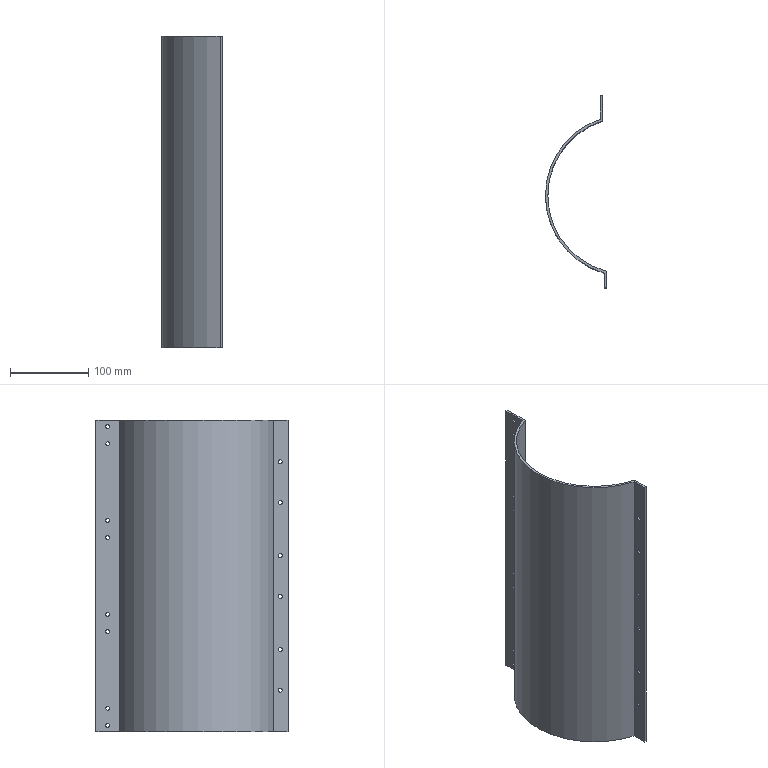Part | SolidWorks | features BaseBody 1 | 1 solid | 39 faces | box 78 x 245.57 x 398 mm | volume 370674 mm3 | cylinder 31 | plane 8 | commonest cylinder face diameters 5 x28 200 x2 206 x1
STEP:
#1=CARTESIAN_POINT('',(-30.,112.57,-365.5));
#2=VERTEX_POINT('',#1);
#3=CARTESIAN_POINT('',(-30.,112.57,-370.5));
#4=VERTEX_POINT('',#3);
#5=CARTESIAN_POINT('',(-30.,112.57,-368.));
#6=DIRECTION('',(-1.,0.,0.));
#7=DIRECTION('',(0.,0.,-1.));
#8=AXIS2_PLACEMENT_3D('',#5,#6,#7);
#9=CIRCLE('',#8,2.5);
#10=EDGE_CURVE('',#2,#4,#9,.T.);
#11=ORIENTED_EDGE('',*,*,#10,.F.);
#12=CARTESIAN_POINT('',(-33.,112.57,-365.5));
#13=VERTEX_POINT('',#12);
#14=CARTESIAN_POINT('',(-33.,112.57,-365.5));
#15=DIRECTION('',(-1.,0.,0.));
#16=VECTOR('',#15,1000.);
#17=LINE('',#14,#16);
#18=EDGE_CURVE('',#2,#13,#17,.T.);
#19=ORIENTED_EDGE('',*,*,#18,.T.);
#20=CARTESIAN_POINT('',(-33.,112.57,-370.5));
#21=VERTEX_POINT('',#20);
#22=CARTESIAN_POINT('',(-33.,112.57,-368.));
#23=DIRECTION('',(1.,0.,0.));
#24=DIRECTION('',(0.,0.,-1.));
#25=AXIS2_PLACEMENT_3D('',#22,#23,#24);
#26=CIRCLE('',#25,2.5);
#27=EDGE_CURVE('',#21,#13,#26,.T.);
#28=ORIENTED_EDGE('',*,*,#27,.F.);
#29=CARTESIAN_POINT('',(-33.,112.57,-370.5));
#30=DIRECTION('',(-1.,0.,0.));
#31=VECTOR('',#30,1000.);
#32=LINE('',#29,#31);
#33=EDGE_CURVE('',#4,#21,#32,.T.);
#34=ORIENTED_EDGE('',*,*,#33,.F.);
#35=EDGE_LOOP('',(#11,#19,#28,#34));
#36=FACE_OUTER_BOUND('',#35,.T.);
#37=CARTESIAN_POINT('',(-33.,112.57,-368.));
#38=DIRECTION('',(-1.,0.,0.));
#39=DIRECTION('',(0.,0.,-1.));
#40=AXIS2_PLACEMENT_3D('',#37,#38,#39);
#41=CYLINDRICAL_SURFACE('',#40,2.5);
#42=ADVANCED_FACE('',(#36),#41,.F.);
#43=CARTESIAN_POINT('',(-30.,112.57,-387.5));
#44=VERTEX_POINT('',#43);
#45=CARTESIAN_POINT('',(-30.,112.57,-392.5));
#46=VERTEX_POINT('',#45);
#47=CARTESIAN_POINT('',(-30.,112.57,-390.));
#48=DIRECTION('',(-1.,0.,0.));
#49=DIRECTION('',(0.,0.,-1.));
#50=AXIS2_PLACEMENT_3D('',#47,#48,#49);
#51=CIRCLE('',#50,2.5);
#52=EDGE_CURVE('',#44,#46,#51,.T.);
#53=ORIENTED_EDGE('',*,*,#52,.F.);
#54=CARTESIAN_POINT('',(-33.,112.57,-387.5));
#55=VERTEX_POINT('',#54);
#56=CARTESIAN_POINT('',(-33.,112.57,-387.5));
#57=DIRECTION('',(-1.,0.,0.));
#58=VECTOR('',#57,1000.);
#59=LINE('',#56,#58);
#60=EDGE_CURVE('',#44,#55,#59,.T.);
#61=ORIENTED_EDGE('',*,*,#60,.T.);
#62=CARTESIAN_POINT('',(-33.,112.57,-392.5));
#63=VERTEX_POINT('',#62);
#64=CARTESIAN_POINT('',(-33.,112.57,-390.));
#65=DIRECTION('',(1.,0.,0.));
#66=DIRECTION('',(0.,0.,-1.));
#67=AXIS2_PLACEMENT_3D('',#64,#65,#66);
#68=CIRCLE('',#67,2.5);
#69=EDGE_CURVE('',#63,#55,#68,.T.);
#70=ORIENTED_EDGE('',*,*,#69,.F.);
#71=CARTESIAN_POINT('',(-33.,112.57,-392.5));
#72=DIRECTION('',(-1.,0.,0.));
#73=VECTOR('',#72,1000.);
#74=LINE('',#71,#73);
#75=EDGE_CURVE('',#46,#63,#74,.T.);
#76=ORIENTED_EDGE('',*,*,#75,.F.);
#77=EDGE_LOOP('',(#53,#61,#70,#76));
#78=FACE_OUTER_BOUND('',#77,.T.);
#79=CARTESIAN_POINT('',(-33.,112.57,-390.));
#80=DIRECTION('',(-1.,0.,0.));
#81=DIRECTION('',(0.,0.,-1.));
#82=AXIS2_PLACEMENT_3D('',#79,#80,#81);
#83=CYLINDRICAL_SURFACE('',#82,2.5);
#84=ADVANCED_FACE('',(#78),#83,.F.);
#85=CARTESIAN_POINT('',(-30.,112.57,-245.5));
#86=VERTEX_POINT('',#85);
#87=CARTESIAN_POINT('',(-30.,112.57,-250.5));
#88=VERTEX_POINT('',#87);
#89=CARTESIAN_POINT('',(-30.,112.57,-248.));
#90=DIRECTION('',(-1.,0.,0.));
#91=DIRECTION('',(0.,0.,-1.));
#92=AXIS2_PLACEMENT_3D('',#89,#90,#91);
#93=CIRCLE('',#92,2.5);
#94=EDGE_CURVE('',#86,#88,#93,.T.);
#95=ORIENTED_EDGE('',*,*,#94,.F.);
#96=CARTESIAN_POINT('',(-33.,112.57,-245.5));
#97=VERTEX_POINT('',#96);
#98=CARTESIAN_POINT('',(-33.,112.57,-245.5));
#99=DIRECTION('',(-1.,0.,0.));
#100=VECTOR('',#99,1000.);
#101=LINE('',#98,#100);
#102=EDGE_CURVE('',#86,#97,#101,.T.);
#103=ORIENTED_EDGE('',*,*,#102,.T.);
#104=CARTESIAN_POINT('',(-33.,112.57,-250.5));
#105=VERTEX_POINT('',#104);
#106=CARTESIAN_POINT('',(-33.,112.57,-248.));
#107=DIRECTION('',(1.,0.,0.));
#108=DIRECTION('',(0.,0.,-1.));
#109=AXIS2_PLACEMENT_3D('',#106,#107,#108);
#110=CIRCLE('',#109,2.5);
#111=EDGE_CURVE('',#105,#97,#110,.T.);
#112=ORIENTED_EDGE('',*,*,#111,.F.);
#113=CARTESIAN_POINT('',(-33.,112.57,-250.5));
#114=DIRECTION('',(-1.,0.,0.));
#115=VECTOR('',#114,1000.);
#116=LINE('',#113,#115);
#117=EDGE_CURVE('',#88,#105,#116,.T.);
#118=ORIENTED_EDGE('',*,*,#117,.F.);
#119=EDGE_LOOP('',(#95,#103,#112,#118));
#120=FACE_OUTER_BOUND('',#119,.T.);
#121=CARTESIAN_POINT('',(-33.,112.57,-248.));
#122=DIRECTION('',(-1.,0.,0.));
#123=DIRECTION('',(0.,0.,-1.));
#124=AXIS2_PLACEMENT_3D('',#121,#122,#123);
#125=CYLINDRICAL_SURFACE('',#124,2.5);
#126=ADVANCED_FACE('',(#120),#125,.F.);
#127=CARTESIAN_POINT('',(-30.,112.57,-267.5));
#128=VERTEX_POINT('',#127);
#129=CARTESIAN_POINT('',(-30.,112.57,-272.5));
#130=VERTEX_POINT('',#129);
#131=CARTESIAN_POINT('',(-30.,112.57,-270.));
#132=DIRECTION('',(-1.,0.,0.));
#133=DIRECTION('',(0.,0.,-1.));
#134=AXIS2_PLACEMENT_3D('',#131,#132,#133);
#135=CIRCLE('',#134,2.5);
#136=EDGE_CURVE('',#128,#130,#135,.T.);
#137=ORIENTED_EDGE('',*,*,#136,.F.);
#138=CARTESIAN_POINT('',(-33.,112.57,-267.5));
#139=VERTEX_POINT('',#138);
#140=CARTESIAN_POINT('',(-33.,112.57,-267.5));
#141=DIRECTION('',(-1.,0.,0.));
#142=VECTOR('',#141,1000.);
#143=LINE('',#140,#142);
#144=EDGE_CURVE('',#128,#139,#143,.T.);
#145=ORIENTED_EDGE('',*,*,#144,.T.);
#146=CARTESIAN_POINT('',(-33.,112.57,-272.5));
#147=VERTEX_POINT('',#146);
#148=CARTESIAN_POINT('',(-33.,112.57,-270.));
#149=DIRECTION('',(1.,0.,0.));
#150=DIRECTION('',(0.,0.,-1.));
#151=AXIS2_PLACEMENT_3D('',#148,#149,#150);
#152=CIRCLE('',#151,2.5);
#153=EDGE_CURVE('',#147,#139,#152,.T.);
#154=ORIENTED_EDGE('',*,*,#153,.F.);
#155=CARTESIAN_POINT('',(-33.,112.57,-272.5));
#156=DIRECTION('',(-1.,0.,0.));
#157=VECTOR('',#156,1000.);
#158=LINE('',#155,#157);
#159=EDGE_CURVE('',#130,#147,#158,.T.);
#160=ORIENTED_EDGE('',*,*,#159,.F.);
#161=EDGE_LOOP('',(#137,#145,#154,#160));
#162=FACE_OUTER_BOUND('',#161,.T.);
#163=CARTESIAN_POINT('',(-33.,112.57,-270.));
#164=DIRECTION('',(-1.,0.,0.));
#165=DIRECTION('',(0.,0.,-1.));
#166=AXIS2_PLACEMENT_3D('',#163,#164,#165);
#167=CYLINDRICAL_SURFACE('',#166,2.5);
#168=ADVANCED_FACE('',(#162),#167,.F.);
#169=CARTESIAN_POINT('',(-30.,112.57,-125.5));
#170=VERTEX_POINT('',#169);
#171=CARTESIAN_POINT('',(-30.,112.57,-130.5));
#172=VERTEX_POINT('',#171);
#173=CARTESIAN_POINT('',(-30.,112.57,-128.));
#174=DIRECTION('',(-1.,0.,0.));
#175=DIRECTION('',(0.,0.,-1.));
#176=AXIS2_PLACEMENT_3D('',#173,#174,#175);
#177=CIRCLE('',#176,2.5);
#178=EDGE_CURVE('',#170,#172,#177,.T.);
#179=ORIENTED_EDGE('',*,*,#178,.F.);
#180=CARTESIAN_POINT('',(-33.,112.57,-125.5));
#181=VERTEX_POINT('',#180);
#182=CARTESIAN_POINT('',(-33.,112.57,-125.5));
#183=DIRECTION('',(-1.,0.,0.));
#184=VECTOR('',#183,1000.);
#185=LINE('',#182,#184);
#186=EDGE_CURVE('',#170,#181,#185,.T.);
#187=ORIENTED_EDGE('',*,*,#186,.T.);
#188=CARTESIAN_POINT('',(-33.,112.57,-130.5));
#189=VERTEX_POINT('',#188);
#190=CARTESIAN_POINT('',(-33.,112.57,-128.));
#191=DIRECTION('',(1.,0.,0.));
#192=DIRECTION('',(0.,0.,-1.));
#193=AXIS2_PLACEMENT_3D('',#190,#191,#192);
#194=CIRCLE('',#193,2.5);
#195=EDGE_CURVE('',#189,#181,#194,.T.);
#196=ORIENTED_EDGE('',*,*,#195,.F.);
#197=CARTESIAN_POINT('',(-33.,112.57,-130.5));
#198=DIRECTION('',(-1.,0.,0.));
#199=VECTOR('',#198,1000.);
#200=LINE('',#197,#199);
#201=EDGE_CURVE('',#172,#189,#200,.T.);
#202=ORIENTED_EDGE('',*,*,#201,.F.);
#203=EDGE_LOOP('',(#179,#187,#196,#202));
#204=FACE_OUTER_BOUND('',#203,.T.);
#205=CARTESIAN_POINT('',(-33.,112.57,-128.));
#206=DIRECTION('',(-1.,0.,0.));
#207=DIRECTION('',(0.,0.,-1.));
#208=AXIS2_PLACEMENT_3D('',#205,#206,#207);
#209=CYLINDRICAL_SURFACE('',#208,2.5);
#210=ADVANCED_FACE('',(#204),#209,.F.);
#211=CARTESIAN_POINT('',(-30.,112.57,-147.5));
#212=VERTEX_POINT('',#211);
#213=CARTESIAN_POINT('',(-30.,112.57,-152.5));
#214=VERTEX_POINT('',#213);
#215=CARTESIAN_POINT('',(-30.,112.57,-150.));
#216=DIRECTION('',(-1.,0.,0.));
#217=DIRECTION('',(0.,0.,-1.));
#218=AXIS2_PLACEMENT_3D('',#215,#216,#217);
#219=CIRCLE('',#218,2.5);
#220=EDGE_CURVE('',#212,#214,#219,.T.);
#221=ORIENTED_EDGE('',*,*,#220,.F.);
#222=CARTESIAN_POINT('',(-33.,112.57,-147.5));
#223=VERTEX_POINT('',#222);
#224=CARTESIAN_POINT('',(-33.,112.57,-147.5));
#225=DIRECTION('',(-1.,0.,0.));
#226=VECTOR('',#225,1000.);
#227=LINE('',#224,#226);
#228=EDGE_CURVE('',#212,#223,#227,.T.);
#229=ORIENTED_EDGE('',*,*,#228,.T.);
#230=CARTESIAN_POINT('',(-33.,112.57,-152.5));
#231=VERTEX_POINT('',#230);
#232=CARTESIAN_POINT('',(-33.,112.57,-150.));
#233=DIRECTION('',(1.,0.,0.));
#234=DIRECTION('',(0.,0.,-1.));
#235=AXIS2_PLACEMENT_3D('',#232,#233,#234);
#236=CIRCLE('',#235,2.5);
#237=EDGE_CURVE('',#231,#223,#236,.T.);
#238=ORIENTED_EDGE('',*,*,#237,.F.);
#239=CARTESIAN_POINT('',(-33.,112.57,-152.5));
#240=DIRECTION('',(-1.,0.,0.));
#241=VECTOR('',#240,1000.);
#242=LINE('',#239,#241);
#243=EDGE_CURVE('',#214,#231,#242,.T.);
#244=ORIENTED_EDGE('',*,*,#243,.F.);
#245=EDGE_LOOP('',(#221,#229,#238,#244));
#246=FACE_OUTER_BOUND('',#245,.T.);
#247=CARTESIAN_POINT('',(-33.,112.57,-150.));
#248=DIRECTION('',(-1.,0.,0.));
#249=DIRECTION('',(0.,0.,-1.));
#250=AXIS2_PLACEMENT_3D('',#247,#248,#249);
#251=CYLINDRICAL_SURFACE('',#250,2.5);
#252=ADVANCED_FACE('',(#246),#251,.F.);
#253=CARTESIAN_POINT('',(-30.,112.57,-5.5));
#254=VERTEX_POINT('',#253);
#255=CARTESIAN_POINT('',(-30.,112.57,-10.5));
#256=VERTEX_POINT('',#255);
#257=CARTESIAN_POINT('',(-30.,112.57,-8.));
#258=DIRECTION('',(-1.,0.,0.));
#259=DIRECTION('',(0.,0.,-1.));
#260=AXIS2_PLACEMENT_3D('',#257,#258,#259);
#261=CIRCLE('',#260,2.5);
#262=EDGE_CURVE('',#254,#256,#261,.T.);
#263=ORIENTED_EDGE('',*,*,#262,.F.);
#264=CARTESIAN_POINT('',(-33.,112.57,-5.5));
#265=VERTEX_POINT('',#264);
#266=CARTESIAN_POINT('',(-33.,112.57,-5.5));
#267=DIRECTION('',(-1.,0.,0.));
#268=VECTOR('',#267,1000.);
#269=LINE('',#266,#268);
#270=EDGE_CURVE('',#254,#265,#269,.T.);
#271=ORIENTED_EDGE('',*,*,#270,.T.);
#272=CARTESIAN_POINT('',(-33.,112.57,-10.5));
#273=VERTEX_POINT('',#272);
#274=CARTESIAN_POINT('',(-33.,112.57,-8.));
#275=DIRECTION('',(1.,0.,0.));
#276=DIRECTION('',(0.,0.,-1.));
#277=AXIS2_PLACEMENT_3D('',#274,#275,#276);
#278=CIRCLE('',#277,2.5);
#279=EDGE_CURVE('',#273,#265,#278,.T.);
#280=ORIENTED_EDGE('',*,*,#279,.F.);
#281=CARTESIAN_POINT('',(-33.,112.57,-10.5));
#282=DIRECTION('',(-1.,0.,0.));
#283=VECTOR('',#282,1000.);
#284=LINE('',#281,#283);
#285=EDGE_CURVE('',#256,#273,#284,.T.);
#286=ORIENTED_EDGE('',*,*,#285,.F.);
#287=EDGE_LOOP('',(#263,#271,#280,#286));
#288=FACE_OUTER_BOUND('',#287,.T.);
#289=CARTESIAN_POINT('',(-33.,112.57,-8.));
#290=DIRECTION('',(-1.,0.,0.));
#291=DIRECTION('',(0.,0.,-1.));
#292=AXIS2_PLACEMENT_3D('',#289,#290,#291);
#293=CYLINDRICAL_SURFACE('',#292,2.5);
#294=ADVANCED_FACE('',(#288),#293,.F.);
#295=CARTESIAN_POINT('',(-30.,112.57,-27.5));
#296=VERTEX_POINT('',#295);
#297=CARTESIAN_POINT('',(-30.,112.57,-32.5));
#298=VERTEX_POINT('',#297);
#299=CARTESIAN_POINT('',(-30.,112.57,-30.));
#300=DIRECTION('',(-1.,0.,0.));
#301=DIRECTION('',(0.,0.,-1.));
#302=AXIS2_PLACEMENT_3D('',#299,#300,#301);
#303=CIRCLE('',#302,2.5);
#304=EDGE_CURVE('',#296,#298,#303,.T.);
#305=ORIENTED_EDGE('',*,*,#304,.F.);
#306=CARTESIAN_POINT('',(-33.,112.57,-27.5));
#307=VERTEX_POINT('',#306);
#308=CARTESIAN_POINT('',(-33.,112.57,-27.5));
#309=DIRECTION('',(-1.,0.,0.));
#310=VECTOR('',#309,1000.);
#311=LINE('',#308,#310);
#312=EDGE_CURVE('',#296,#307,#311,.T.);
#313=ORIENTED_EDGE('',*,*,#312,.T.);
#314=CARTESIAN_POINT('',(-33.,112.57,-32.5));
#315=VERTEX_POINT('',#314);
#316=CARTESIAN_POINT('',(-33.,112.57,-30.));
#317=DIRECTION('',(1.,0.,0.));
#318=DIRECTION('',(0.,0.,-1.));
#319=AXIS2_PLACEMENT_3D('',#316,#317,#318);
#320=CIRCLE('',#319,2.5);
#321=EDGE_CURVE('',#315,#307,#320,.T.);
#322=ORIENTED_EDGE('',*,*,#321,.F.);
#323=CARTESIAN_POINT('',(-33.,112.57,-32.5));
#324=DIRECTION('',(-1.,0.,0.));
#325=VECTOR('',#324,1000.);
#326=LINE('',#323,#325);
#327=EDGE_CURVE('',#298,#315,#326,.T.);
#328=ORIENTED_EDGE('',*,*,#327,.F.);
#329=EDGE_LOOP('',(#305,#313,#322,#328));
#330=FACE_OUTER_BOUND('',#329,.T.);
#331=CARTESIAN_POINT('',(-33.,112.57,-30.));
#332=DIRECTION('',(-1.,0.,0.));
#333=DIRECTION('',(0.,0.,-1.));
#334=AXIS2_PLACEMENT_3D('',#331,#332,#333);
#335=CYLINDRICAL_SURFACE('',#334,2.5);
#336=ADVANCED_FACE('',(#330),#335,.F.);
#337=CARTESIAN_POINT('',(-25.,-108.,-290.5));
#338=VERTEX_POINT('',#337);
#339=CARTESIAN_POINT('',(-25.,-108.,-295.5));
#340=VERTEX_POINT('',#339);
#341=CARTESIAN_POINT('',(-25.,-108.,-293.));
#342=DIRECTION('',(-1.,0.,0.));
#343=DIRECTION('',(0.,0.,-1.));
#344=AXIS2_PLACEMENT_3D('',#341,#342,#343);
#345=CIRCLE('',#344,2.5);
#346=EDGE_CURVE('',#338,#340,#345,.T.);
#347=ORIENTED_EDGE('',*,*,#346,.F.);
#348=CARTESIAN_POINT('',(-28.,-108.,-290.5));
#349=VERTEX_POINT('',#348);
#350=CARTESIAN_POINT('',(-28.,-108.,-290.5));
#351=DIRECTION('',(-1.,0.,0.));
#352=VECTOR('',#351,1000.);
#353=LINE('',#350,#352);
#354=EDGE_CURVE('',#338,#349,#353,.T.);
#355=ORIENTED_EDGE('',*,*,#354,.T.);
#356=CARTESIAN_POINT('',(-28.,-108.,-295.5));
#357=VERTEX_POINT('',#356);
#358=CARTESIAN_POINT('',(-28.,-108.,-293.));
#359=DIRECTION('',(1.,0.,0.));
#360=DIRECTION('',(0.,0.,-1.));
#361=AXIS2_PLACEMENT_3D('',#358,#359,#360);
#362=CIRCLE('',#361,2.5);
#363=EDGE_CURVE('',#357,#349,#362,.T.);
#364=ORIENTED_EDGE('',*,*,#363,.F.);
#365=CARTESIAN_POINT('',(-28.,-108.,-295.5));
#366=DIRECTION('',(-1.,0.,0.));
#367=VECTOR('',#366,1000.);
#368=LINE('',#365,#367);
#369=EDGE_CURVE('',#340,#357,#368,.T.);
#370=ORIENTED_EDGE('',*,*,#369,.F.);
#371=EDGE_LOOP('',(#347,#355,#364,#370));
#372=FACE_OUTER_BOUND('',#371,.T.);
#373=CARTESIAN_POINT('',(-28.,-108.,-293.));
#374=DIRECTION('',(-1.,0.,0.));
#375=DIRECTION('',(0.,0.,-1.));
#376=AXIS2_PLACEMENT_3D('',#373,#374,#375);
#377=CYLINDRICAL_SURFACE('',#376,2.5);
#378=ADVANCED_FACE('',(#372),#377,.F.);
#379=CARTESIAN_POINT('',(-25.,-108.,-342.5));
#380=VERTEX_POINT('',#379);
#381=CARTESIAN_POINT('',(-25.,-108.,-347.5));
#382=VERTEX_POINT('',#381);
#383=CARTESIAN_POINT('',(-25.,-108.,-345.));
#384=DIRECTION('',(-1.,0.,0.));
#385=DIRECTION('',(0.,0.,-1.));
#386=AXIS2_PLACEMENT_3D('',#383,#384,#385);
#387=CIRCLE('',#386,2.5);
#388=EDGE_CURVE('',#380,#382,#387,.T.);
#389=ORIENTED_EDGE('',*,*,#388,.F.);
#390=CARTESIAN_POINT('',(-28.,-108.,-342.5));
#391=VERTEX_POINT('',#390);
#392=CARTESIAN_POINT('',(-28.,-108.,-342.5));
#393=DIRECTION('',(-1.,0.,0.));
#394=VECTOR('',#393,1000.);
#395=LINE('',#392,#394);
#396=EDGE_CURVE('',#380,#391,#395,.T.);
#397=ORIENTED_EDGE('',*,*,#396,.T.);
#398=CARTESIAN_POINT('',(-28.,-108.,-347.5));
#399=VERTEX_POINT('',#398);
#400=CARTESIAN_POINT('',(-28.,-108.,-345.));
#401=DIRECTION('',(1.,0.,0.));
#402=DIRECTION('',(0.,0.,-1.));
#403=AXIS2_PLACEMENT_3D('',#400,#401,#402);
#404=CIRCLE('',#403,2.5);
#405=EDGE_CURVE('',#399,#391,#404,.T.);
#406=ORIENTED_EDGE('',*,*,#405,.F.);
#407=CARTESIAN_POINT('',(-28.,-108.,-347.5));
#408=DIRECTION('',(-1.,0.,0.));
#409=VECTOR('',#408,1000.);
#410=LINE('',#407,#409);
#411=EDGE_CURVE('',#382,#399,#410,.T.);
#412=ORIENTED_EDGE('',*,*,#411,.F.);
#413=EDGE_LOOP('',(#389,#397,#406,#412));
#414=FACE_OUTER_BOUND('',#413,.T.);
#415=CARTESIAN_POINT('',(-28.,-108.,-345.));
#416=DIRECTION('',(-1.,0.,0.));
#417=DIRECTION('',(0.,0.,-1.));
#418=AXIS2_PLACEMENT_3D('',#415,#416,#417);
#419=CYLINDRICAL_SURFACE('',#418,2.5);
#420=ADVANCED_FACE('',(#414),#419,.F.);
#421=CARTESIAN_POINT('',(-25.,-108.,-170.5));
#422=VERTEX_POINT('',#421);
#423=CARTESIAN_POINT('',(-25.,-108.,-175.5));
#424=VERTEX_POINT('',#423);
#425=CARTESIAN_POINT('',(-25.,-108.,-173.));
#426=DIRECTION('',(-1.,0.,0.));
#427=DIRECTION('',(0.,0.,-1.));
#428=AXIS2_PLACEMENT_3D('',#425,#426,#427);
#429=CIRCLE('',#428,2.5);
#430=EDGE_CURVE('',#422,#424,#429,.T.);
#431=ORIENTED_EDGE('',*,*,#430,.F.);
#432=CARTESIAN_POINT('',(-28.,-108.,-170.5));
#433=VERTEX_POINT('',#432);
#434=CARTESIAN_POINT('',(-28.,-108.,-170.5));
#435=DIRECTION('',(-1.,0.,0.));
#436=VECTOR('',#435,1000.);
#437=LINE('',#434,#436);
#438=EDGE_CURVE('',#422,#433,#437,.T.);
#439=ORIENTED_EDGE('',*,*,#438,.T.);
#440=CARTESIAN_POINT('',(-28.,-108.,-175.5));
#441=VERTEX_POINT('',#440);
#442=CARTESIAN_POINT('',(-28.,-108.,-173.));
#443=DIRECTION('',(1.,0.,0.));
#444=DIRECTION('',(0.,0.,-1.));
#445=AXIS2_PLACEMENT_3D('',#442,#443,#444);
#446=CIRCLE('',#445,2.5);
#447=EDGE_CURVE('',#441,#433,#446,.T.);
#448=ORIENTED_EDGE('',*,*,#447,.F.);
#449=CARTESIAN_POINT('',(-28.,-108.,-175.5));
#450=DIRECTION('',(-1.,0.,0.));
#451=VECTOR('',#450,1000.);
#452=LINE('',#449,#451);
#453=EDGE_CURVE('',#424,#441,#452,.T.);
#454=ORIENTED_EDGE('',*,*,#453,.F.);
#455=EDGE_LOOP('',(#431,#439,#448,#454));
#456=FACE_OUTER_BOUND('',#455,.T.);
#457=CARTESIAN_POINT('',(-28.,-108.,-173.));
#458=DIRECTION('',(-1.,0.,0.));
#459=DIRECTION('',(0.,0.,-1.));
#460=AXIS2_PLACEMENT_3D('',#457,#458,#459);
#461=CYLINDRICAL_SURFACE('',#460,2.5);
#462=ADVANCED_FACE('',(#456),#461,.F.);
#463=CARTESIAN_POINT('',(-25.,-108.,-222.5));
#464=VERTEX_POINT('',#463);
#465=CARTESIAN_POINT('',(-25.,-108.,-227.5));
#466=VERTEX_POINT('',#465);
#467=CARTESIAN_POINT('',(-25.,-108.,-225.));
#468=DIRECTION('',(-1.,0.,0.));
#469=DIRECTION('',(0.,0.,-1.));
#470=AXIS2_PLACEMENT_3D('',#467,#468,#469);
#471=CIRCLE('',#470,2.5);
#472=EDGE_CURVE('',#464,#466,#471,.T.);
#473=ORIENTED_EDGE('',*,*,#472,.F.);
#474=CARTESIAN_POINT('',(-28.,-108.,-222.5));
#475=VERTEX_POINT('',#474);
#476=CARTESIAN_POINT('',(-28.,-108.,-222.5));
#477=DIRECTION('',(-1.,0.,0.));
#478=VECTOR('',#477,1000.);
#479=LINE('',#476,#478);
#480=EDGE_CURVE('',#464,#475,#479,.T.);
#481=ORIENTED_EDGE('',*,*,#480,.T.);
#482=CARTESIAN_POINT('',(-28.,-108.,-227.5));
#483=VERTEX_POINT('',#482);
#484=CARTESIAN_POINT('',(-28.,-108.,-225.));
#485=DIRECTION('',(1.,0.,0.));
#486=DIRECTION('',(0.,0.,-1.));
#487=AXIS2_PLACEMENT_3D('',#484,#485,#486);
#488=CIRCLE('',#487,2.5);
#489=EDGE_CURVE('',#483,#475,#488,.T.);
#490=ORIENTED_EDGE('',*,*,#489,.F.);
#491=CARTESIAN_POINT('',(-28.,-108.,-227.5));
#492=DIRECTION('',(-1.,0.,0.));
#493=VECTOR('',#492,1000.);
#494=LINE('',#491,#493);
#495=EDGE_CURVE('',#466,#483,#494,.T.);
#496=ORIENTED_EDGE('',*,*,#495,.F.);
#497=EDGE_LOOP('',(#473,#481,#490,#496));
#498=FACE_OUTER_BOUND('',#497,.T.);
#499=CARTESIAN_POINT('',(-28.,-108.,-225.));
#500=DIRECTION('',(-1.,0.,0.));
#501=DIRECTION('',(0.,0.,-1.));
#502=AXIS2_PLACEMENT_3D('',#499,#500,#501);
#503=CYLINDRICAL_SURFACE('',#502,2.5);
#504=ADVANCED_FACE('',(#498),#503,.F.);
#505=CARTESIAN_POINT('',(-25.,-108.,-50.5));
#506=VERTEX_POINT('',#505);
#507=CARTESIAN_POINT('',(-25.,-108.,-55.5));
#508=VERTEX_POINT('',#507);
#509=CARTESIAN_POINT('',(-25.,-108.,-53.));
#510=DIRECTION('',(-1.,0.,0.));
#511=DIRECTION('',(0.,0.,-1.));
#512=AXIS2_PLACEMENT_3D('',#509,#510,#511);
#513=CIRCLE('',#512,2.5);
#514=EDGE_CURVE('',#506,#508,#513,.T.);
#515=ORIENTED_EDGE('',*,*,#514,.F.);
#516=CARTESIAN_POINT('',(-28.,-108.,-50.5));
#517=VERTEX_POINT('',#516);
#518=CARTESIAN_POINT('',(-28.,-108.,-50.5));
#519=DIRECTION('',(-1.,0.,0.));
#520=VECTOR('',#519,1000.);
#521=LINE('',#518,#520);
#522=EDGE_CURVE('',#506,#517,#521,.T.);
#523=ORIENTED_EDGE('',*,*,#522,.T.);
#524=CARTESIAN_POINT('',(-28.,-108.,-55.5));
#525=VERTEX_POINT('',#524);
#526=CARTESIAN_POINT('',(-28.,-108.,-53.));
#527=DIRECTION('',(1.,0.,0.));
#528=DIRECTION('',(0.,0.,-1.));
#529=AXIS2_PLACEMENT_3D('',#526,#527,#528);
#530=CIRCLE('',#529,2.5);
#531=EDGE_CURVE('',#525,#517,#530,.T.);
#532=ORIENTED_EDGE('',*,*,#531,.F.);
#533=CARTESIAN_POINT('',(-28.,-108.,-55.5));
#534=DIRECTION('',(-1.,0.,0.));
#535=VECTOR('',#534,1000.);
#536=LINE('',#533,#535);
#537=EDGE_CURVE('',#508,#525,#536,.T.);
#538=ORIENTED_EDGE('',*,*,#537,.F.);
#539=EDGE_LOOP('',(#515,#523,#532,#538));
#540=FACE_OUTER_BOUND('',#539,.T.);
#541=CARTESIAN_POINT('',(-28.,-108.,-53.));
#542=DIRECTION('',(-1.,0.,0.));
#543=DIRECTION('',(0.,0.,-1.));
#544=AXIS2_PLACEMENT_3D('',#541,#542,#543);
#545=CYLINDRICAL_SURFACE('',#544,2.5);
#546=ADVANCED_FACE('',(#540),#545,.F.);
#547=CARTESIAN_POINT('',(-25.,-108.,-102.5));
#548=VERTEX_POINT('',#547);
#549=CARTESIAN_POINT('',(-25.,-108.,-107.5));
#550=VERTEX_POINT('',#549);
#551=CARTESIAN_POINT('',(-25.,-108.,-105.));
#552=DIRECTION('',(-1.,0.,0.));
#553=DIRECTION('',(0.,0.,-1.));
#554=AXIS2_PLACEMENT_3D('',#551,#552,#553);
#555=CIRCLE('',#554,2.5);
#556=EDGE_CURVE('',#548,#550,#555,.T.);
#557=ORIENTED_EDGE('',*,*,#556,.F.);
#558=CARTESIAN_POINT('',(-28.,-108.,-102.5));
#559=VERTEX_POINT('',#558);
#560=CARTESIAN_POINT('',(-28.,-108.,-102.5));
#561=DIRECTION('',(-1.,0.,0.));
#562=VECTOR('',#561,1000.);
#563=LINE('',#560,#562);
#564=EDGE_CURVE('',#548,#559,#563,.T.);
#565=ORIENTED_EDGE('',*,*,#564,.T.);
#566=CARTESIAN_POINT('',(-28.,-108.,-107.5));
#567=VERTEX_POINT('',#566);
#568=CARTESIAN_POINT('',(-28.,-108.,-105.));
#569=DIRECTION('',(1.,0.,0.));
#570=DIRECTION('',(0.,0.,-1.));
#571=AXIS2_PLACEMENT_3D('',#568,#569,#570);
#572=CIRCLE('',#571,2.5);
#573=EDGE_CURVE('',#567,#559,#572,.T.);
#574=ORIENTED_EDGE('',*,*,#573,.F.);
#575=CARTESIAN_POINT('',(-28.,-108.,-107.5));
#576=DIRECTION('',(-1.,0.,0.));
#577=VECTOR('',#576,1000.);
#578=LINE('',#575,#577);
#579=EDGE_CURVE('',#550,#567,#578,.T.);
#580=ORIENTED_EDGE('',*,*,#579,.F.);
#581=EDGE_LOOP('',(#557,#565,#574,#580));
#582=FACE_OUTER_BOUND('',#581,.T.);
#583=CARTESIAN_POINT('',(-28.,-108.,-105.));
#584=DIRECTION('',(-1.,0.,0.));
#585=DIRECTION('',(0.,0.,-1.));
#586=AXIS2_PLACEMENT_3D('',#583,#584,#585);
#587=CYLINDRICAL_SURFACE('',#586,2.5);
#588=ADVANCED_FACE('',(#582),#587,.F.);
#589=CARTESIAN_POINT('',(-100.,0.,-398.));
#590=VERTEX_POINT('',#589);
#591=CARTESIAN_POINT('',(-25.,-96.825,-398.));
#592=VERTEX_POINT('',#591);
#593=CARTESIAN_POINT('',(0.,0.,-398.));
#594=DIRECTION('',(0.,0.,1.));
#595=DIRECTION('',(-1.,0.,0.));
#596=AXIS2_PLACEMENT_3D('',#593,#594,#595);
#597=CIRCLE('',#596,100.);
#598=EDGE_CURVE('',#590,#592,#597,.T.);
#599=ORIENTED_EDGE('',*,*,#598,.F.);
#600=CARTESIAN_POINT('',(-100.,0.,0.));
#601=VERTEX_POINT('',#600);
#602=CARTESIAN_POINT('',(-100.,0.,0.));
#603=DIRECTION('',(0.,0.,1.));
#604=VECTOR('',#603,1000.);
#605=LINE('',#602,#604);
#606=EDGE_CURVE('',#590,#601,#605,.T.);
#607=ORIENTED_EDGE('',*,*,#606,.T.);
#608=CARTESIAN_POINT('',(-25.,-96.825,0.));
#609=VERTEX_POINT('',#608);
#610=CARTESIAN_POINT('',(0.,0.,0.));
#611=DIRECTION('',(0.,0.,-1.));
#612=DIRECTION('',(-1.,0.,0.));
#613=AXIS2_PLACEMENT_3D('',#610,#611,#612);
#614=CIRCLE('',#613,100.);
#615=EDGE_CURVE('',#609,#601,#614,.T.);
#616=ORIENTED_EDGE('',*,*,#615,.F.);
#617=CARTESIAN_POINT('',(-25.,-96.825,0.));
#618=DIRECTION('',(0.,0.,-1.));
#619=VECTOR('',#618,1000.);
#620=LINE('',#617,#619);
#621=EDGE_CURVE('',#609,#592,#620,.T.);
#622=ORIENTED_EDGE('',*,*,#621,.T.);
#623=EDGE_LOOP('',(#599,#607,#616,#622));
#624=FACE_OUTER_BOUND('',#623,.T.);
#625=CARTESIAN_POINT('',(0.,0.,0.));
#626=DIRECTION('',(0.,0.,1.));
#627=DIRECTION('',(-1.,0.,0.));
#628=AXIS2_PLACEMENT_3D('',#625,#626,#627);
#629=CYLINDRICAL_SURFACE('',#628,100.);
#630=ADVANCED_FACE('',(#624),#629,.F.);
#631=CARTESIAN_POINT('',(-30.,112.57,-368.));
#632=DIRECTION('',(-1.,0.,0.));
#633=DIRECTION('',(0.,0.,-1.));
#634=AXIS2_PLACEMENT_3D('',#631,#632,#633);
#635=CIRCLE('',#634,2.5);
#636=EDGE_CURVE('',#4,#2,#635,.T.);
#637=ORIENTED_EDGE('',*,*,#636,.T.);
#638=ORIENTED_EDGE('',*,*,#10,.T.);
#639=EDGE_LOOP('',(#637,#638));
#640=FACE_BOUND('',#639,.T.);
#641=CARTESIAN_POINT('',(-30.,112.57,-390.));
#642=DIRECTION('',(-1.,0.,0.));
#643=DIRECTION('',(0.,0.,-1.));
#644=AXIS2_PLACEMENT_3D('',#641,#642,#643);
#645=CIRCLE('',#644,2.5);
#646=EDGE_CURVE('',#46,#44,#645,.T.);
#647=ORIENTED_EDGE('',*,*,#646,.T.);
#648=ORIENTED_EDGE('',*,*,#52,.T.);
#649=EDGE_LOOP('',(#647,#648));
#650=FACE_BOUND('',#649,.T.);
#651=CARTESIAN_POINT('',(-30.,112.57,-248.));
#652=DIRECTION('',(-1.,0.,0.));
#653=DIRECTION('',(0.,0.,-1.));
#654=AXIS2_PLACEMENT_3D('',#651,#652,#653);
#655=CIRCLE('',#654,2.5);
#656=EDGE_CURVE('',#88,#86,#655,.T.);
#657=ORIENTED_EDGE('',*,*,#656,.T.);
#658=ORIENTED_EDGE('',*,*,#94,.T.);
#659=EDGE_LOOP('',(#657,#658));
#660=FACE_BOUND('',#659,.T.);
#661=CARTESIAN_POINT('',(-30.,112.57,-270.));
#662=DIRECTION('',(-1.,0.,0.));
#663=DIRECTION('',(0.,0.,-1.));
#664=AXIS2_PLACEMENT_3D('',#661,#662,#663);
#665=CIRCLE('',#664,2.5);
#666=EDGE_CURVE('',#130,#128,#665,.T.);
#667=ORIENTED_EDGE('',*,*,#666,.T.);
#668=ORIENTED_EDGE('',*,*,#136,.T.);
#669=EDGE_LOOP('',(#667,#668));
#670=FACE_BOUND('',#669,.T.);
#671=CARTESIAN_POINT('',(-30.,112.57,-128.));
#672=DIRECTION('',(-1.,0.,0.));
#673=DIRECTION('',(0.,0.,-1.));
#674=AXIS2_PLACEMENT_3D('',#671,#672,#673);
#675=CIRCLE('',#674,2.5);
#676=EDGE_CURVE('',#172,#170,#675,.T.);
#677=ORIENTED_EDGE('',*,*,#676,.T.);
#678=ORIENTED_EDGE('',*,*,#178,.T.);
#679=EDGE_LOOP('',(#677,#678));
#680=FACE_BOUND('',#679,.T.);
#681=CARTESIAN_POINT('',(-30.,112.57,-150.));
#682=DIRECTION('',(-1.,0.,0.));
#683=DIRECTION('',(0.,0.,-1.));
#684=AXIS2_PLACEMENT_3D('',#681,#682,#683);
#685=CIRCLE('',#684,2.5);
#686=EDGE_CURVE('',#214,#212,#685,.T.);
#687=ORIENTED_EDGE('',*,*,#686,.T.);
#688=ORIENTED_EDGE('',*,*,#220,.T.);
#689=EDGE_LOOP('',(#687,#688));
#690=FACE_BOUND('',#689,.T.);
#691=CARTESIAN_POINT('',(-30.,112.57,-8.));
#692=DIRECTION('',(-1.,0.,0.));
#693=DIRECTION('',(0.,0.,-1.));
#694=AXIS2_PLACEMENT_3D('',#691,#692,#693);
#695=CIRCLE('',#694,2.5);
#696=EDGE_CURVE('',#256,#254,#695,.T.);
#697=ORIENTED_EDGE('',*,*,#696,.T.);
#698=ORIENTED_EDGE('',*,*,#262,.T.);
#699=EDGE_LOOP('',(#697,#698));
#700=FACE_BOUND('',#699,.T.);
#701=CARTESIAN_POINT('',(-30.,112.57,-30.));
#702=DIRECTION('',(-1.,0.,0.));
#703=DIRECTION('',(0.,0.,-1.));
#704=AXIS2_PLACEMENT_3D('',#701,#702,#703);
#705=CIRCLE('',#704,2.5);
#706=EDGE_CURVE('',#298,#296,#705,.T.);
#707=ORIENTED_EDGE('',*,*,#706,.T.);
#708=ORIENTED_EDGE('',*,*,#304,.T.);
#709=EDGE_LOOP('',(#707,#708));
#710=FACE_BOUND('',#709,.T.);
#711=CARTESIAN_POINT('',(-30.,95.394,0.));
#712=VERTEX_POINT('',#711);
#713=CARTESIAN_POINT('',(-30.,127.57,0.));
#714=VERTEX_POINT('',#713);
#715=CARTESIAN_POINT('',(-30.,95.394,0.));
#716=DIRECTION('',(0.,1.,0.));
#717=VECTOR('',#716,1000.);
#718=LINE('',#715,#717);
#719=EDGE_CURVE('',#712,#714,#718,.T.);
#720=ORIENTED_EDGE('',*,*,#719,.F.);
#721=CARTESIAN_POINT('',(-30.,95.394,-398.));
#722=VERTEX_POINT('',#721);
#723=CARTESIAN_POINT('',(-30.,95.394,0.));
#724=DIRECTION('',(0.,0.,-1.));
#725=VECTOR('',#724,1000.);
#726=LINE('',#723,#725);
#727=EDGE_CURVE('',#712,#722,#726,.T.);
#728=ORIENTED_EDGE('',*,*,#727,.T.);
#729=CARTESIAN_POINT('',(-30.,127.57,-398.));
#730=VERTEX_POINT('',#729);
#731=CARTESIAN_POINT('',(-30.,95.394,-398.));
#732=DIRECTION('',(0.,-1.,0.));
#733=VECTOR('',#732,1000.);
#734=LINE('',#731,#733);
#735=EDGE_CURVE('',#730,#722,#734,.T.);
#736=ORIENTED_EDGE('',*,*,#735,.F.);
#737=CARTESIAN_POINT('',(-30.,127.57,0.));
#738=DIRECTION('',(0.,0.,-1.));
#739=VECTOR('',#738,1000.);
#740=LINE('',#737,#739);
#741=EDGE_CURVE('',#714,#730,#740,.T.);
#742=ORIENTED_EDGE('',*,*,#741,.F.);
#743=EDGE_LOOP('',(#720,#728,#736,#742));
#744=FACE_OUTER_BOUND('',#743,.T.);
#745=CARTESIAN_POINT('',(-30.,127.57,0.));
#746=DIRECTION('',(1.,0.,0.));
#747=DIRECTION('',(0.,1.,0.));
#748=AXIS2_PLACEMENT_3D('',#745,#746,#747);
#749=PLANE('',#748);
#750=ADVANCED_FACE('',(#640,#650,#660,#670,#680,#690,#700,#710,#744),#749,.T.);
#751=CARTESIAN_POINT('',(-33.,127.57,0.));
#752=VERTEX_POINT('',#751);
#753=CARTESIAN_POINT('',(-30.,127.57,0.));
#754=DIRECTION('',(-1.,0.,0.));
#755=VECTOR('',#754,1000.);
#756=LINE('',#753,#755);
#757=EDGE_CURVE('',#714,#752,#756,.T.);
#758=ORIENTED_EDGE('',*,*,#757,.F.);
#759=ORIENTED_EDGE('',*,*,#741,.T.);
#760=CARTESIAN_POINT('',(-33.,127.57,-398.));
#761=VERTEX_POINT('',#760);
#762=CARTESIAN_POINT('',(-30.,127.57,-398.));
#763=DIRECTION('',(1.,0.,0.));
#764=VECTOR('',#763,1000.);
#765=LINE('',#762,#764);
#766=EDGE_CURVE('',#761,#730,#765,.T.);
#767=ORIENTED_EDGE('',*,*,#766,.F.);
#768=CARTESIAN_POINT('',(-33.,127.57,0.));
#769=DIRECTION('',(0.,0.,-1.));
#770=VECTOR('',#769,1000.);
#771=LINE('',#768,#770);
#772=EDGE_CURVE('',#752,#761,#771,.T.);
#773=ORIENTED_EDGE('',*,*,#772,.F.);
#774=EDGE_LOOP('',(#758,#759,#767,#773));
#775=FACE_OUTER_BOUND('',#774,.T.);
#776=CARTESIAN_POINT('',(-33.,127.57,0.));
#777=DIRECTION('',(0.,1.,0.));
#778=DIRECTION('',(1.,0.,0.));
#779=AXIS2_PLACEMENT_3D('',#776,#777,#778);
#780=PLANE('',#779);
#781=ADVANCED_FACE('',(#775),#780,.T.);
#782=ORIENTED_EDGE('',*,*,#27,.T.);
#783=CARTESIAN_POINT('',(-33.,112.57,-368.));
#784=DIRECTION('',(1.,0.,0.));
#785=DIRECTION('',(0.,0.,-1.));
#786=AXIS2_PLACEMENT_3D('',#783,#784,#785);
#787=CIRCLE('',#786,2.5);
#788=EDGE_CURVE('',#13,#21,#787,.T.);
#789=ORIENTED_EDGE('',*,*,#788,.T.);
#790=EDGE_LOOP('',(#782,#789));
#791=FACE_BOUND('',#790,.T.);
#792=ORIENTED_EDGE('',*,*,#69,.T.);
#793=CARTESIAN_POINT('',(-33.,112.57,-390.));
#794=DIRECTION('',(1.,0.,0.));
#795=DIRECTION('',(0.,0.,-1.));
#796=AXIS2_PLACEMENT_3D('',#793,#794,#795);
#797=CIRCLE('',#796,2.5);
#798=EDGE_CURVE('',#55,#63,#797,.T.);
#799=ORIENTED_EDGE('',*,*,#798,.T.);
#800=EDGE_LOOP('',(#792,#799));
#801=FACE_BOUND('',#800,.T.);
#802=ORIENTED_EDGE('',*,*,#111,.T.);
#803=CARTESIAN_POINT('',(-33.,112.57,-248.));
#804=DIRECTION('',(1.,0.,0.));
#805=DIRECTION('',(0.,0.,-1.));
#806=AXIS2_PLACEMENT_3D('',#803,#804,#805);
#807=CIRCLE('',#806,2.5);
#808=EDGE_CURVE('',#97,#105,#807,.T.);
#809=ORIENTED_EDGE('',*,*,#808,.T.);
#810=EDGE_LOOP('',(#802,#809));
#811=FACE_BOUND('',#810,.T.);
#812=ORIENTED_EDGE('',*,*,#153,.T.);
#813=CARTESIAN_POINT('',(-33.,112.57,-270.));
#814=DIRECTION('',(1.,0.,0.));
#815=DIRECTION('',(0.,0.,-1.));
#816=AXIS2_PLACEMENT_3D('',#813,#814,#815);
#817=CIRCLE('',#816,2.5);
#818=EDGE_CURVE('',#139,#147,#817,.T.);
#819=ORIENTED_EDGE('',*,*,#818,.T.);
#820=EDGE_LOOP('',(#812,#819));
#821=FACE_BOUND('',#820,.T.);
#822=ORIENTED_EDGE('',*,*,#195,.T.);
#823=CARTESIAN_POINT('',(-33.,112.57,-128.));
#824=DIRECTION('',(1.,0.,0.));
#825=DIRECTION('',(0.,0.,-1.));
#826=AXIS2_PLACEMENT_3D('',#823,#824,#825);
#827=CIRCLE('',#826,2.5);
#828=EDGE_CURVE('',#181,#189,#827,.T.);
#829=ORIENTED_EDGE('',*,*,#828,.T.);
#830=EDGE_LOOP('',(#822,#829));
#831=FACE_BOUND('',#830,.T.);
#832=ORIENTED_EDGE('',*,*,#237,.T.);
#833=CARTESIAN_POINT('',(-33.,112.57,-150.));
#834=DIRECTION('',(1.,0.,0.));
#835=DIRECTION('',(0.,0.,-1.));
#836=AXIS2_PLACEMENT_3D('',#833,#834,#835);
#837=CIRCLE('',#836,2.5);
#838=EDGE_CURVE('',#223,#231,#837,.T.);
#839=ORIENTED_EDGE('',*,*,#838,.T.);
#840=EDGE_LOOP('',(#832,#839));
#841=FACE_BOUND('',#840,.T.);
#842=ORIENTED_EDGE('',*,*,#279,.T.);
#843=CARTESIAN_POINT('',(-33.,112.57,-8.));
#844=DIRECTION('',(1.,0.,0.));
#845=DIRECTION('',(0.,0.,-1.));
#846=AXIS2_PLACEMENT_3D('',#843,#844,#845);
#847=CIRCLE('',#846,2.5);
#848=EDGE_CURVE('',#265,#273,#847,.T.);
#849=ORIENTED_EDGE('',*,*,#848,.T.);
#850=EDGE_LOOP('',(#842,#849));
#851=FACE_BOUND('',#850,.T.);
#852=ORIENTED_EDGE('',*,*,#321,.T.);
#853=CARTESIAN_POINT('',(-33.,112.57,-30.));
#854=DIRECTION('',(1.,0.,0.));
#855=DIRECTION('',(0.,0.,-1.));
#856=AXIS2_PLACEMENT_3D('',#853,#854,#855);
#857=CIRCLE('',#856,2.5);
#858=EDGE_CURVE('',#307,#315,#857,.T.);
#859=ORIENTED_EDGE('',*,*,#858,.T.);
#860=EDGE_LOOP('',(#852,#859));
#861=FACE_BOUND('',#860,.T.);
#862=CARTESIAN_POINT('',(-33.,97.57,0.));
#863=VERTEX_POINT('',#862);
#864=CARTESIAN_POINT('',(-33.,127.57,0.));
#865=DIRECTION('',(0.,-1.,0.));
#866=VECTOR('',#865,1000.);
#867=LINE('',#864,#866);
#868=EDGE_CURVE('',#752,#863,#867,.T.);
#869=ORIENTED_EDGE('',*,*,#868,.F.);
#870=ORIENTED_EDGE('',*,*,#772,.T.);
#871=CARTESIAN_POINT('',(-33.,97.57,-398.));
#872=VERTEX_POINT('',#871);
#873=CARTESIAN_POINT('',(-33.,127.57,-398.));
#874=DIRECTION('',(0.,1.,0.));
#875=VECTOR('',#874,1000.);
#876=LINE('',#873,#875);
#877=EDGE_CURVE('',#872,#761,#876,.T.);
#878=ORIENTED_EDGE('',*,*,#877,.F.);
#879=CARTESIAN_POINT('',(-33.,97.57,0.));
#880=DIRECTION('',(0.,0.,-1.));
#881=VECTOR('',#880,1000.);
#882=LINE('',#879,#881);
#883=EDGE_CURVE('',#863,#872,#882,.T.);
#884=ORIENTED_EDGE('',*,*,#883,.F.);
#885=EDGE_LOOP('',(#869,#870,#878,#884));
#886=FACE_OUTER_BOUND('',#885,.T.);
#887=CARTESIAN_POINT('',(-33.,97.57,0.));
#888=DIRECTION('',(-1.,0.,0.));
#889=DIRECTION('',(0.,1.,0.));
#890=AXIS2_PLACEMENT_3D('',#887,#888,#889);
#891=PLANE('',#890);
#892=ADVANCED_FACE('',(#791,#801,#811,#821,#831,#841,#851,#861,#886),#891,.T.);
#893=CARTESIAN_POINT('',(-28.,-99.121,0.));
#894=VERTEX_POINT('',#893);
#895=CARTESIAN_POINT('',(0.,0.,0.));
#896=DIRECTION('',(0.,0.,1.));
#897=DIRECTION('',(-0.3204,0.9473,0.));
#898=AXIS2_PLACEMENT_3D('',#895,#896,#897);
#899=CIRCLE('',#898,103.);
#900=EDGE_CURVE('',#863,#894,#899,.T.);
#901=ORIENTED_EDGE('',*,*,#900,.F.);
#902=ORIENTED_EDGE('',*,*,#883,.T.);
#903=CARTESIAN_POINT('',(-28.,-99.121,-398.));
#904=VERTEX_POINT('',#903);
#905=CARTESIAN_POINT('',(0.,0.,-398.));
#906=DIRECTION('',(0.,0.,-1.));
#907=DIRECTION('',(-0.3204,0.9473,0.));
#908=AXIS2_PLACEMENT_3D('',#905,#906,#907);
#909=CIRCLE('',#908,103.);
#910=EDGE_CURVE('',#904,#872,#909,.T.);
#911=ORIENTED_EDGE('',*,*,#910,.F.);
#912=CARTESIAN_POINT('',(-28.,-99.121,0.));
#913=DIRECTION('',(0.,0.,-1.));
#914=VECTOR('',#913,1000.);
#915=LINE('',#912,#914);
#916=EDGE_CURVE('',#894,#904,#915,.T.);
#917=ORIENTED_EDGE('',*,*,#916,.F.);
#918=EDGE_LOOP('',(#901,#902,#911,#917));
#919=FACE_OUTER_BOUND('',#918,.T.);
#920=CARTESIAN_POINT('',(0.,0.,0.));
#921=DIRECTION('',(0.,0.,1.));
#922=DIRECTION('',(-0.3204,0.9473,0.));
#923=AXIS2_PLACEMENT_3D('',#920,#921,#922);
#924=CYLINDRICAL_SURFACE('',#923,103.);
#925=ADVANCED_FACE('',(#919),#924,.T.);
#926=ORIENTED_EDGE('',*,*,#363,.T.);
#927=CARTESIAN_POINT('',(-28.,-108.,-293.));
#928=DIRECTION('',(1.,0.,0.));
#929=DIRECTION('',(0.,0.,-1.));
#930=AXIS2_PLACEMENT_3D('',#927,#928,#929);
#931=CIRCLE('',#930,2.5);
#932=EDGE_CURVE('',#349,#357,#931,.T.);
#933=ORIENTED_EDGE('',*,*,#932,.T.);
#934=EDGE_LOOP('',(#926,#933));
#935=FACE_BOUND('',#934,.T.);
#936=ORIENTED_EDGE('',*,*,#405,.T.);
#937=CARTESIAN_POINT('',(-28.,-108.,-345.));
#938=DIRECTION('',(1.,0.,0.));
#939=DIRECTION('',(0.,0.,-1.));
#940=AXIS2_PLACEMENT_3D('',#937,#938,#939);
#941=CIRCLE('',#940,2.5);
#942=EDGE_CURVE('',#391,#399,#941,.T.);
#943=ORIENTED_EDGE('',*,*,#942,.T.);
#944=EDGE_LOOP('',(#936,#943));
#945=FACE_BOUND('',#944,.T.);
#946=ORIENTED_EDGE('',*,*,#447,.T.);
#947=CARTESIAN_POINT('',(-28.,-108.,-173.));
#948=DIRECTION('',(1.,0.,0.));
#949=DIRECTION('',(0.,0.,-1.));
#950=AXIS2_PLACEMENT_3D('',#947,#948,#949);
#951=CIRCLE('',#950,2.5);
#952=EDGE_CURVE('',#433,#441,#951,.T.);
#953=ORIENTED_EDGE('',*,*,#952,.T.);
#954=EDGE_LOOP('',(#946,#953));
#955=FACE_BOUND('',#954,.T.);
#956=ORIENTED_EDGE('',*,*,#489,.T.);
#957=CARTESIAN_POINT('',(-28.,-108.,-225.));
#958=DIRECTION('',(1.,0.,0.));
#959=DIRECTION('',(0.,0.,-1.));
#960=AXIS2_PLACEMENT_3D('',#957,#958,#959);
#961=CIRCLE('',#960,2.5);
#962=EDGE_CURVE('',#475,#483,#961,.T.);
#963=ORIENTED_EDGE('',*,*,#962,.T.);
#964=EDGE_LOOP('',(#956,#963));
#965=FACE_BOUND('',#964,.T.);
#966=ORIENTED_EDGE('',*,*,#531,.T.);
#967=CARTESIAN_POINT('',(-28.,-108.,-53.));
#968=DIRECTION('',(1.,0.,0.));
#969=DIRECTION('',(0.,0.,-1.));
#970=AXIS2_PLACEMENT_3D('',#967,#968,#969);
#971=CIRCLE('',#970,2.5);
#972=EDGE_CURVE('',#517,#525,#971,.T.);
#973=ORIENTED_EDGE('',*,*,#972,.T.);
#974=EDGE_LOOP('',(#966,#973));
#975=FACE_BOUND('',#974,.T.);
#976=ORIENTED_EDGE('',*,*,#573,.T.);
#977=CARTESIAN_POINT('',(-28.,-108.,-105.));
#978=DIRECTION('',(1.,0.,0.));
#979=DIRECTION('',(0.,0.,-1.));
#980=AXIS2_PLACEMENT_3D('',#977,#978,#979);
#981=CIRCLE('',#980,2.5);
#982=EDGE_CURVE('',#559,#567,#981,.T.);
#983=ORIENTED_EDGE('',*,*,#982,.T.);
#984=EDGE_LOOP('',(#976,#983));
#985=FACE_BOUND('',#984,.T.);
#986=CARTESIAN_POINT('',(-28.,-118.,0.));
#987=VERTEX_POINT('',#986);
#988=CARTESIAN_POINT('',(-28.,-99.121,0.));
#989=DIRECTION('',(0.,-1.,0.));
#990=VECTOR('',#989,1000.);
#991=LINE('',#988,#990);
#992=EDGE_CURVE('',#894,#987,#991,.T.);
#993=ORIENTED_EDGE('',*,*,#992,.F.);
#994=ORIENTED_EDGE('',*,*,#916,.T.);
#995=CARTESIAN_POINT('',(-28.,-118.,-398.));
#996=VERTEX_POINT('',#995);
#997=CARTESIAN_POINT('',(-28.,-99.121,-398.));
#998=DIRECTION('',(0.,1.,0.));
#999=VECTOR('',#998,1000.);
#1000=LINE('',#997,#999);
#1001=EDGE_CURVE('',#996,#904,#1000,.T.);
#1002=ORIENTED_EDGE('',*,*,#1001,.F.);
#1003=CARTESIAN_POINT('',(-28.,-118.,0.));
#1004=DIRECTION('',(0.,0.,-1.));
#1005=VECTOR('',#1004,1000.);
#1006=LINE('',#1003,#1005);
#1007=EDGE_CURVE('',#987,#996,#1006,.T.);
#1008=ORIENTED_EDGE('',*,*,#1007,.F.);
#1009=EDGE_LOOP('',(#993,#994,#1002,#1008));
#1010=FACE_OUTER_BOUND('',#1009,.T.);
#1011=CARTESIAN_POINT('',(-28.,-118.,0.));
#1012=DIRECTION('',(-1.,0.,0.));
#1013=DIRECTION('',(0.,0.,1.));
#1014=AXIS2_PLACEMENT_3D('',#1011,#1012,#1013);
#1015=PLANE('',#1014);
#1016=ADVANCED_FACE('',(#935,#945,#955,#965,#975,#985,#1010),#1015,.T.);
#1017=CARTESIAN_POINT('',(-25.,-118.,0.));
#1018=VERTEX_POINT('',#1017);
#1019=CARTESIAN_POINT('',(-28.,-118.,0.));
#1020=DIRECTION('',(1.,0.,0.));
#1021=VECTOR('',#1020,1000.);
#1022=LINE('',#1019,#1021);
#1023=EDGE_CURVE('',#987,#1018,#1022,.T.);
#1024=ORIENTED_EDGE('',*,*,#1023,.F.);
#1025=ORIENTED_EDGE('',*,*,#1007,.T.);
#1026=CARTESIAN_POINT('',(-25.,-118.,-398.));
#1027=VERTEX_POINT('',#1026);
#1028=CARTESIAN_POINT('',(-28.,-118.,-398.));
#1029=DIRECTION('',(-1.,0.,0.));
#1030=VECTOR('',#1029,1000.);
#1031=LINE('',#1028,#1030);
#1032=EDGE_CURVE('',#1027,#996,#1031,.T.);
#1033=ORIENTED_EDGE('',*,*,#1032,.F.);
#1034=CARTESIAN_POINT('',(-25.,-118.,0.));
#1035=DIRECTION('',(0.,0.,-1.));
#1036=VECTOR('',#1035,1000.);
#1037=LINE('',#1034,#1036);
#1038=EDGE_CURVE('',#1018,#1027,#1037,.T.);
#1039=ORIENTED_EDGE('',*,*,#1038,.F.);
#1040=EDGE_LOOP('',(#1024,#1025,#1033,#1039));
#1041=FACE_OUTER_BOUND('',#1040,.T.);
#1042=CARTESIAN_POINT('',(-25.,-118.,0.));
#1043=DIRECTION('',(0.,-1.,0.));
#1044=DIRECTION('',(0.,0.,-1.));
#1045=AXIS2_PLACEMENT_3D('',#1042,#1043,#1044);
#1046=PLANE('',#1045);
#1047=ADVANCED_FACE('',(#1041),#1046,.T.);
#1048=CARTESIAN_POINT('',(-25.,-108.,-293.));
#1049=DIRECTION('',(-1.,0.,0.));
#1050=DIRECTION('',(0.,0.,-1.));
#1051=AXIS2_PLACEMENT_3D('',#1048,#1049,#1050);
#1052=CIRCLE('',#1051,2.5);
#1053=EDGE_CURVE('',#340,#338,#1052,.T.);
#1054=ORIENTED_EDGE('',*,*,#1053,.T.);
#1055=ORIENTED_EDGE('',*,*,#346,.T.);
#1056=EDGE_LOOP('',(#1054,#1055));
#1057=FACE_BOUND('',#1056,.T.);
#1058=CARTESIAN_POINT('',(-25.,-108.,-345.));
#1059=DIRECTION('',(-1.,0.,0.));
#1060=DIRECTION('',(0.,0.,-1.));
#1061=AXIS2_PLACEMENT_3D('',#1058,#1059,#1060);
#1062=CIRCLE('',#1061,2.5);
#1063=EDGE_CURVE('',#382,#380,#1062,.T.);
#1064=ORIENTED_EDGE('',*,*,#1063,.T.);
#1065=ORIENTED_EDGE('',*,*,#388,.T.);
#1066=EDGE_LOOP('',(#1064,#1065));
#1067=FACE_BOUND('',#1066,.T.);
#1068=CARTESIAN_POINT('',(-25.,-108.,-173.));
#1069=DIRECTION('',(-1.,0.,0.));
#1070=DIRECTION('',(0.,0.,-1.));
#1071=AXIS2_PLACEMENT_3D('',#1068,#1069,#1070);
#1072=CIRCLE('',#1071,2.5);
#1073=EDGE_CURVE('',#424,#422,#1072,.T.);
#1074=ORIENTED_EDGE('',*,*,#1073,.T.);
#1075=ORIENTED_EDGE('',*,*,#430,.T.);
#1076=EDGE_LOOP('',(#1074,#1075));
#1077=FACE_BOUND('',#1076,.T.);
#1078=CARTESIAN_POINT('',(-25.,-108.,-225.));
#1079=DIRECTION('',(-1.,0.,0.));
#1080=DIRECTION('',(0.,0.,-1.));
#1081=AXIS2_PLACEMENT_3D('',#1078,#1079,#1080);
#1082=CIRCLE('',#1081,2.5);
#1083=EDGE_CURVE('',#466,#464,#1082,.T.);
#1084=ORIENTED_EDGE('',*,*,#1083,.T.);
#1085=ORIENTED_EDGE('',*,*,#472,.T.);
#1086=EDGE_LOOP('',(#1084,#1085));
#1087=FACE_BOUND('',#1086,.T.);
#1088=CARTESIAN_POINT('',(-25.,-108.,-53.));
#1089=DIRECTION('',(-1.,0.,0.));
#1090=DIRECTION('',(0.,0.,-1.));
#1091=AXIS2_PLACEMENT_3D('',#1088,#1089,#1090);
#1092=CIRCLE('',#1091,2.5);
#1093=EDGE_CURVE('',#508,#506,#1092,.T.);
#1094=ORIENTED_EDGE('',*,*,#1093,.T.);
#1095=ORIENTED_EDGE('',*,*,#514,.T.);
#1096=EDGE_LOOP('',(#1094,#1095));
#1097=FACE_BOUND('',#1096,.T.);
#1098=CARTESIAN_POINT('',(-25.,-108.,-105.));
#1099=DIRECTION('',(-1.,0.,0.));
#1100=DIRECTION('',(0.,0.,-1.));
#1101=AXIS2_PLACEMENT_3D('',#1098,#1099,#1100);
#1102=CIRCLE('',#1101,2.5);
#1103=EDGE_CURVE('',#550,#548,#1102,.T.);
#1104=ORIENTED_EDGE('',*,*,#1103,.T.);
#1105=ORIENTED_EDGE('',*,*,#556,.T.);
#1106=EDGE_LOOP('',(#1104,#1105));
#1107=FACE_BOUND('',#1106,.T.);
#1108=CARTESIAN_POINT('',(-25.,-118.,0.));
#1109=DIRECTION('',(0.,1.,0.));
#1110=VECTOR('',#1109,1000.);
#1111=LINE('',#1108,#1110);
#1112=EDGE_CURVE('',#1018,#609,#1111,.T.);
#1113=ORIENTED_EDGE('',*,*,#1112,.F.);
#1114=ORIENTED_EDGE('',*,*,#1038,.T.);
#1115=CARTESIAN_POINT('',(-25.,-118.,-398.));
#1116=DIRECTION('',(0.,-1.,0.));
#1117=VECTOR('',#1116,1000.);
#1118=LINE('',#1115,#1117);
#1119=EDGE_CURVE('',#592,#1027,#1118,.T.);
#1120=ORIENTED_EDGE('',*,*,#1119,.F.);
#1121=ORIENTED_EDGE('',*,*,#621,.F.);
#1122=EDGE_LOOP('',(#1113,#1114,#1120,#1121));
#1123=FACE_OUTER_BOUND('',#1122,.T.);
#1124=CARTESIAN_POINT('',(-25.,-96.825,0.));
#1125=DIRECTION('',(1.,0.,0.));
#1126=DIRECTION('',(0.,-1.,0.));
#1127=AXIS2_PLACEMENT_3D('',#1124,#1125,#1126);
#1128=PLANE('',#1127);
#1129=ADVANCED_FACE('',(#1057,#1067,#1077,#1087,#1097,#1107,#1123),#1128,.T.);
#1130=ORIENTED_EDGE('',*,*,#615,.T.);
#1131=CARTESIAN_POINT('',(0.,0.,0.));
#1132=DIRECTION('',(0.,0.,-1.));
#1133=DIRECTION('',(-1.,0.,0.));
#1134=AXIS2_PLACEMENT_3D('',#1131,#1132,#1133);
#1135=CIRCLE('',#1134,100.);
#1136=EDGE_CURVE('',#601,#712,#1135,.T.);
#1137=ORIENTED_EDGE('',*,*,#1136,.T.);
#1138=ORIENTED_EDGE('',*,*,#719,.T.);
#1139=ORIENTED_EDGE('',*,*,#757,.T.);
#1140=ORIENTED_EDGE('',*,*,#868,.T.);
#1141=ORIENTED_EDGE('',*,*,#900,.T.);
#1142=ORIENTED_EDGE('',*,*,#992,.T.);
#1143=ORIENTED_EDGE('',*,*,#1023,.T.);
#1144=ORIENTED_EDGE('',*,*,#1112,.T.);
#1145=EDGE_LOOP('',(#1130,#1137,#1138,#1139,#1140,#1141,#1142,#1143,#1144));
#1146=FACE_OUTER_BOUND('',#1145,.T.);
#1147=CARTESIAN_POINT('',(-65.824,3.829,0.));
#1148=DIRECTION('',(0.,0.,1.));
#1149=DIRECTION('',(1.,0.,0.));
#1150=AXIS2_PLACEMENT_3D('',#1147,#1148,#1149);
#1151=PLANE('',#1150);
#1152=ADVANCED_FACE('',(#1146),#1151,.T.);
#1153=ORIENTED_EDGE('',*,*,#735,.T.);
#1154=CARTESIAN_POINT('',(0.,0.,-398.));
#1155=DIRECTION('',(0.,0.,1.));
#1156=DIRECTION('',(-1.,0.,0.));
#1157=AXIS2_PLACEMENT_3D('',#1154,#1155,#1156);
#1158=CIRCLE('',#1157,100.);
#1159=EDGE_CURVE('',#722,#590,#1158,.T.);
#1160=ORIENTED_EDGE('',*,*,#1159,.T.);
#1161=ORIENTED_EDGE('',*,*,#598,.T.);
#1162=ORIENTED_EDGE('',*,*,#1119,.T.);
#1163=ORIENTED_EDGE('',*,*,#1032,.T.);
#1164=ORIENTED_EDGE('',*,*,#1001,.T.);
#1165=ORIENTED_EDGE('',*,*,#910,.T.);
#1166=ORIENTED_EDGE('',*,*,#877,.T.);
#1167=ORIENTED_EDGE('',*,*,#766,.T.);
#1168=EDGE_LOOP('',(#1153,#1160,#1161,#1162,#1163,#1164,#1165,#1166,#1167));
#1169=FACE_OUTER_BOUND('',#1168,.T.);
#1170=CARTESIAN_POINT('',(-65.824,3.829,-398.));
#1171=DIRECTION('',(0.,0.,1.));
#1172=DIRECTION('',(1.,0.,0.));
#1173=AXIS2_PLACEMENT_3D('',#1170,#1171,#1172);
#1174=PLANE('',#1173);
#1175=ADVANCED_FACE('',(#1169),#1174,.F.);
#1176=ORIENTED_EDGE('',*,*,#606,.F.);
#1177=ORIENTED_EDGE('',*,*,#1159,.F.);
#1178=ORIENTED_EDGE('',*,*,#727,.F.);
#1179=ORIENTED_EDGE('',*,*,#1136,.F.);
#1180=EDGE_LOOP('',(#1176,#1177,#1178,#1179));
#1181=FACE_OUTER_BOUND('',#1180,.T.);
#1182=CARTESIAN_POINT('',(0.,0.,0.));
#1183=DIRECTION('',(0.,0.,1.));
#1184=DIRECTION('',(-1.,0.,0.));
#1185=AXIS2_PLACEMENT_3D('',#1182,#1183,#1184);
#1186=CYLINDRICAL_SURFACE('',#1185,100.);
#1187=ADVANCED_FACE('',(#1181),#1186,.F.);
#1188=ORIENTED_EDGE('',*,*,#564,.F.);
#1189=ORIENTED_EDGE('',*,*,#1103,.F.);
#1190=ORIENTED_EDGE('',*,*,#579,.T.);
#1191=ORIENTED_EDGE('',*,*,#982,.F.);
#1192=EDGE_LOOP('',(#1188,#1189,#1190,#1191));
#1193=FACE_OUTER_BOUND('',#1192,.T.);
#1194=CARTESIAN_POINT('',(-28.,-108.,-105.));
#1195=DIRECTION('',(-1.,0.,0.));
#1196=DIRECTION('',(0.,0.,-1.));
#1197=AXIS2_PLACEMENT_3D('',#1194,#1195,#1196);
#1198=CYLINDRICAL_SURFACE('',#1197,2.5);
#1199=ADVANCED_FACE('',(#1193),#1198,.F.);
#1200=ORIENTED_EDGE('',*,*,#522,.F.);
#1201=ORIENTED_EDGE('',*,*,#1093,.F.);
#1202=ORIENTED_EDGE('',*,*,#537,.T.);
#1203=ORIENTED_EDGE('',*,*,#972,.F.);
#1204=EDGE_LOOP('',(#1200,#1201,#1202,#1203));
#1205=FACE_OUTER_BOUND('',#1204,.T.);
#1206=CARTESIAN_POINT('',(-28.,-108.,-53.));
#1207=DIRECTION('',(-1.,0.,0.));
#1208=DIRECTION('',(0.,0.,-1.));
#1209=AXIS2_PLACEMENT_3D('',#1206,#1207,#1208);
#1210=CYLINDRICAL_SURFACE('',#1209,2.5);
#1211=ADVANCED_FACE('',(#1205),#1210,.F.);
#1212=ORIENTED_EDGE('',*,*,#480,.F.);
#1213=ORIENTED_EDGE('',*,*,#1083,.F.);
#1214=ORIENTED_EDGE('',*,*,#495,.T.);
#1215=ORIENTED_EDGE('',*,*,#962,.F.);
#1216=EDGE_LOOP('',(#1212,#1213,#1214,#1215));
#1217=FACE_OUTER_BOUND('',#1216,.T.);
#1218=CARTESIAN_POINT('',(-28.,-108.,-225.));
#1219=DIRECTION('',(-1.,0.,0.));
#1220=DIRECTION('',(0.,0.,-1.));
#1221=AXIS2_PLACEMENT_3D('',#1218,#1219,#1220);
#1222=CYLINDRICAL_SURFACE('',#1221,2.5);
#1223=ADVANCED_FACE('',(#1217),#1222,.F.);
#1224=ORIENTED_EDGE('',*,*,#438,.F.);
#1225=ORIENTED_EDGE('',*,*,#1073,.F.);
#1226=ORIENTED_EDGE('',*,*,#453,.T.);
#1227=ORIENTED_EDGE('',*,*,#952,.F.);
#1228=EDGE_LOOP('',(#1224,#1225,#1226,#1227));
#1229=FACE_OUTER_BOUND('',#1228,.T.);
#1230=CARTESIAN_POINT('',(-28.,-108.,-173.));
#1231=DIRECTION('',(-1.,0.,0.));
#1232=DIRECTION('',(0.,0.,-1.));
#1233=AXIS2_PLACEMENT_3D('',#1230,#1231,#1232);
#1234=CYLINDRICAL_SURFACE('',#1233,2.5);
#1235=ADVANCED_FACE('',(#1229),#1234,.F.);
#1236=ORIENTED_EDGE('',*,*,#396,.F.);
#1237=ORIENTED_EDGE('',*,*,#1063,.F.);
#1238=ORIENTED_EDGE('',*,*,#411,.T.);
#1239=ORIENTED_EDGE('',*,*,#942,.F.);
#1240=EDGE_LOOP('',(#1236,#1237,#1238,#1239));
#1241=FACE_OUTER_BOUND('',#1240,.T.);
#1242=CARTESIAN_POINT('',(-28.,-108.,-345.));
#1243=DIRECTION('',(-1.,0.,0.));
#1244=DIRECTION('',(0.,0.,-1.));
#1245=AXIS2_PLACEMENT_3D('',#1242,#1243,#1244);
#1246=CYLINDRICAL_SURFACE('',#1245,2.5);
#1247=ADVANCED_FACE('',(#1241),#1246,.F.);
#1248=ORIENTED_EDGE('',*,*,#354,.F.);
#1249=ORIENTED_EDGE('',*,*,#1053,.F.);
#1250=ORIENTED_EDGE('',*,*,#369,.T.);
#1251=ORIENTED_EDGE('',*,*,#932,.F.);
#1252=EDGE_LOOP('',(#1248,#1249,#1250,#1251));
#1253=FACE_OUTER_BOUND('',#1252,.T.);
#1254=CARTESIAN_POINT('',(-28.,-108.,-293.));
#1255=DIRECTION('',(-1.,0.,0.));
#1256=DIRECTION('',(0.,0.,-1.));
#1257=AXIS2_PLACEMENT_3D('',#1254,#1255,#1256);
#1258=CYLINDRICAL_SURFACE('',#1257,2.5);
#1259=ADVANCED_FACE('',(#1253),#1258,.F.);
#1260=ORIENTED_EDGE('',*,*,#312,.F.);
#1261=ORIENTED_EDGE('',*,*,#706,.F.);
#1262=ORIENTED_EDGE('',*,*,#327,.T.);
#1263=ORIENTED_EDGE('',*,*,#858,.F.);
#1264=EDGE_LOOP('',(#1260,#1261,#1262,#1263));
#1265=FACE_OUTER_BOUND('',#1264,.T.);
#1266=CARTESIAN_POINT('',(-33.,112.57,-30.));
#1267=DIRECTION('',(-1.,0.,0.));
#1268=DIRECTION('',(0.,0.,-1.));
#1269=AXIS2_PLACEMENT_3D('',#1266,#1267,#1268);
#1270=CYLINDRICAL_SURFACE('',#1269,2.5);
#1271=ADVANCED_FACE('',(#1265),#1270,.F.);
#1272=ORIENTED_EDGE('',*,*,#270,.F.);
#1273=ORIENTED_EDGE('',*,*,#696,.F.);
#1274=ORIENTED_EDGE('',*,*,#285,.T.);
#1275=ORIENTED_EDGE('',*,*,#848,.F.);
#1276=EDGE_LOOP('',(#1272,#1273,#1274,#1275));
#1277=FACE_OUTER_BOUND('',#1276,.T.);
#1278=CARTESIAN_POINT('',(-33.,112.57,-8.));
#1279=DIRECTION('',(-1.,0.,0.));
#1280=DIRECTION('',(0.,0.,-1.));
#1281=AXIS2_PLACEMENT_3D('',#1278,#1279,#1280);
#1282=CYLINDRICAL_SURFACE('',#1281,2.5);
#1283=ADVANCED_FACE('',(#1277),#1282,.F.);
#1284=ORIENTED_EDGE('',*,*,#228,.F.);
#1285=ORIENTED_EDGE('',*,*,#686,.F.);
#1286=ORIENTED_EDGE('',*,*,#243,.T.);
#1287=ORIENTED_EDGE('',*,*,#838,.F.);
#1288=EDGE_LOOP('',(#1284,#1285,#1286,#1287));
#1289=FACE_OUTER_BOUND('',#1288,.T.);
#1290=CARTESIAN_POINT('',(-33.,112.57,-150.));
#1291=DIRECTION('',(-1.,0.,0.));
#1292=DIRECTION('',(0.,0.,-1.));
#1293=AXIS2_PLACEMENT_3D('',#1290,#1291,#1292);
#1294=CYLINDRICAL_SURFACE('',#1293,2.5);
#1295=ADVANCED_FACE('',(#1289),#1294,.F.);
#1296=ORIENTED_EDGE('',*,*,#186,.F.);
#1297=ORIENTED_EDGE('',*,*,#676,.F.);
#1298=ORIENTED_EDGE('',*,*,#201,.T.);
#1299=ORIENTED_EDGE('',*,*,#828,.F.);
#1300=EDGE_LOOP('',(#1296,#1297,#1298,#1299));
#1301=FACE_OUTER_BOUND('',#1300,.T.);
#1302=CARTESIAN_POINT('',(-33.,112.57,-128.));
#1303=DIRECTION('',(-1.,0.,0.));
#1304=DIRECTION('',(0.,0.,-1.));
#1305=AXIS2_PLACEMENT_3D('',#1302,#1303,#1304);
#1306=CYLINDRICAL_SURFACE('',#1305,2.5);
#1307=ADVANCED_FACE('',(#1301),#1306,.F.);
#1308=ORIENTED_EDGE('',*,*,#144,.F.);
#1309=ORIENTED_EDGE('',*,*,#666,.F.);
#1310=ORIENTED_EDGE('',*,*,#159,.T.);
#1311=ORIENTED_EDGE('',*,*,#818,.F.);
#1312=EDGE_LOOP('',(#1308,#1309,#1310,#1311));
#1313=FACE_OUTER_BOUND('',#1312,.T.);
#1314=CARTESIAN_POINT('',(-33.,112.57,-270.));
#1315=DIRECTION('',(-1.,0.,0.));
#1316=DIRECTION('',(0.,0.,-1.));
#1317=AXIS2_PLACEMENT_3D('',#1314,#1315,#1316);
#1318=CYLINDRICAL_SURFACE('',#1317,2.5);
#1319=ADVANCED_FACE('',(#1313),#1318,.F.);
#1320=ORIENTED_EDGE('',*,*,#102,.F.);
#1321=ORIENTED_EDGE('',*,*,#656,.F.);
#1322=ORIENTED_EDGE('',*,*,#117,.T.);
#1323=ORIENTED_EDGE('',*,*,#808,.F.);
#1324=EDGE_LOOP('',(#1320,#1321,#1322,#1323));
#1325=FACE_OUTER_BOUND('',#1324,.T.);
#1326=CARTESIAN_POINT('',(-33.,112.57,-248.));
#1327=DIRECTION('',(-1.,0.,0.));
#1328=DIRECTION('',(0.,0.,-1.));
#1329=AXIS2_PLACEMENT_3D('',#1326,#1327,#1328);
#1330=CYLINDRICAL_SURFACE('',#1329,2.5);
#1331=ADVANCED_FACE('',(#1325),#1330,.F.);
#1332=ORIENTED_EDGE('',*,*,#60,.F.);
#1333=ORIENTED_EDGE('',*,*,#646,.F.);
#1334=ORIENTED_EDGE('',*,*,#75,.T.);
#1335=ORIENTED_EDGE('',*,*,#798,.F.);
#1336=EDGE_LOOP('',(#1332,#1333,#1334,#1335));
#1337=FACE_OUTER_BOUND('',#1336,.T.);
#1338=CARTESIAN_POINT('',(-33.,112.57,-390.));
#1339=DIRECTION('',(-1.,0.,0.));
#1340=DIRECTION('',(0.,0.,-1.));
#1341=AXIS2_PLACEMENT_3D('',#1338,#1339,#1340);
#1342=CYLINDRICAL_SURFACE('',#1341,2.5);
#1343=ADVANCED_FACE('',(#1337),#1342,.F.);
#1344=ORIENTED_EDGE('',*,*,#18,.F.);
#1345=ORIENTED_EDGE('',*,*,#636,.F.);
#1346=ORIENTED_EDGE('',*,*,#33,.T.);
#1347=ORIENTED_EDGE('',*,*,#788,.F.);
#1348=EDGE_LOOP('',(#1344,#1345,#1346,#1347));
#1349=FACE_OUTER_BOUND('',#1348,.T.);
#1350=CARTESIAN_POINT('',(-33.,112.57,-368.));
#1351=DIRECTION('',(-1.,0.,0.));
#1352=DIRECTION('',(0.,0.,-1.));
#1353=AXIS2_PLACEMENT_3D('',#1350,#1351,#1352);
#1354=CYLINDRICAL_SURFACE('',#1353,2.5);
#1355=ADVANCED_FACE('',(#1349),#1354,.F.);
#1356=CLOSED_SHELL('',(#42,#84,#126,#168,#210,#252,#294,#336,#378,#420,#462,#504,#546,#588,#630,#750,#781,#892,#925,#1016,#1047,#1129,#1152,#1175,#1187,#1199,#1211,#1223,#1235,#1247,#1259,#1271,#1283,#1295,#1307,#1319,#1331,#1343,#1355));
#1357=MANIFOLD_SOLID_BREP('',#1356);
#1358=CARTESIAN_POINT('',(0.,0.,0.));
#1359=DIRECTION('',(0.,0.,1.));
#1360=DIRECTION('',(1.,0.,0.));
#1361=AXIS2_PLACEMENT_3D('',#1358,#1359,#1360);
#1362=(LENGTH_UNIT()NAMED_UNIT(*)SI_UNIT(.MILLI.,.METRE.));
#1363=UNCERTAINTY_MEASURE_WITH_UNIT(LENGTH_MEASURE(0.00001),#1362,'','');
#1364=(NAMED_UNIT(*)PLANE_ANGLE_UNIT()SI_UNIT($,.RADIAN.));
#1365=(NAMED_UNIT(*)SI_UNIT($,.STERADIAN.)SOLID_ANGLE_UNIT());
#1366=(GEOMETRIC_REPRESENTATION_CONTEXT(3)GLOBAL_UNCERTAINTY_ASSIGNED_CONTEXT((#1363))GLOBAL_UNIT_ASSIGNED_CONTEXT((#1362,#1364,#1365))REPRESENTATION_CONTEXT('',''));
#1367=ADVANCED_BREP_SHAPE_REPRESENTATION('',(#1357,#1361),#1366);